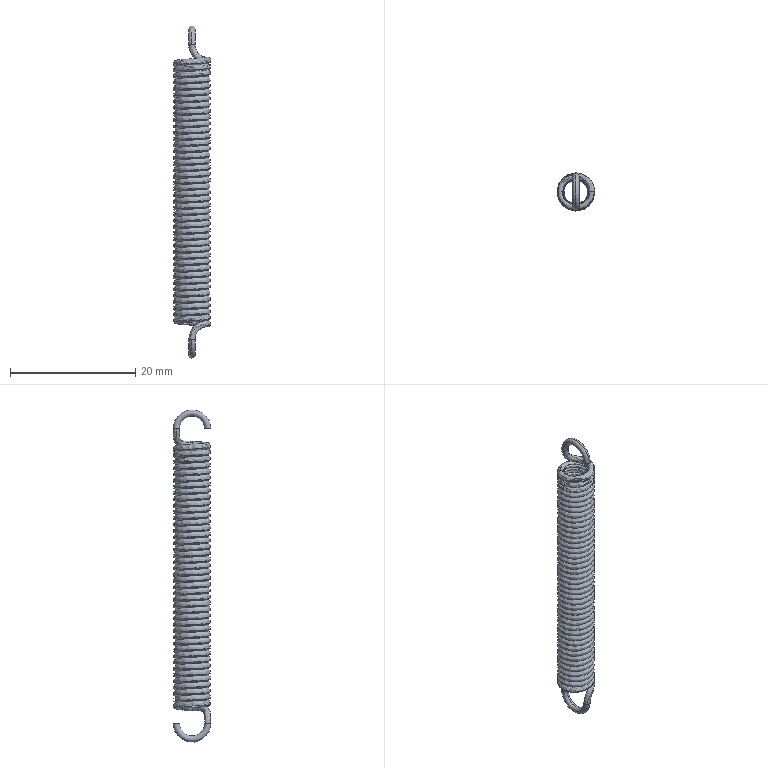Part | SolidWorks | features RefCurve 2, CompositeCurve 1, Helix 1, Sweep 1 | 1 solid | 12 faces | box 5.989 x 6.003 x 53 mm | volume 518.141 mm3 | spline 6 | torus 4 | plane 2